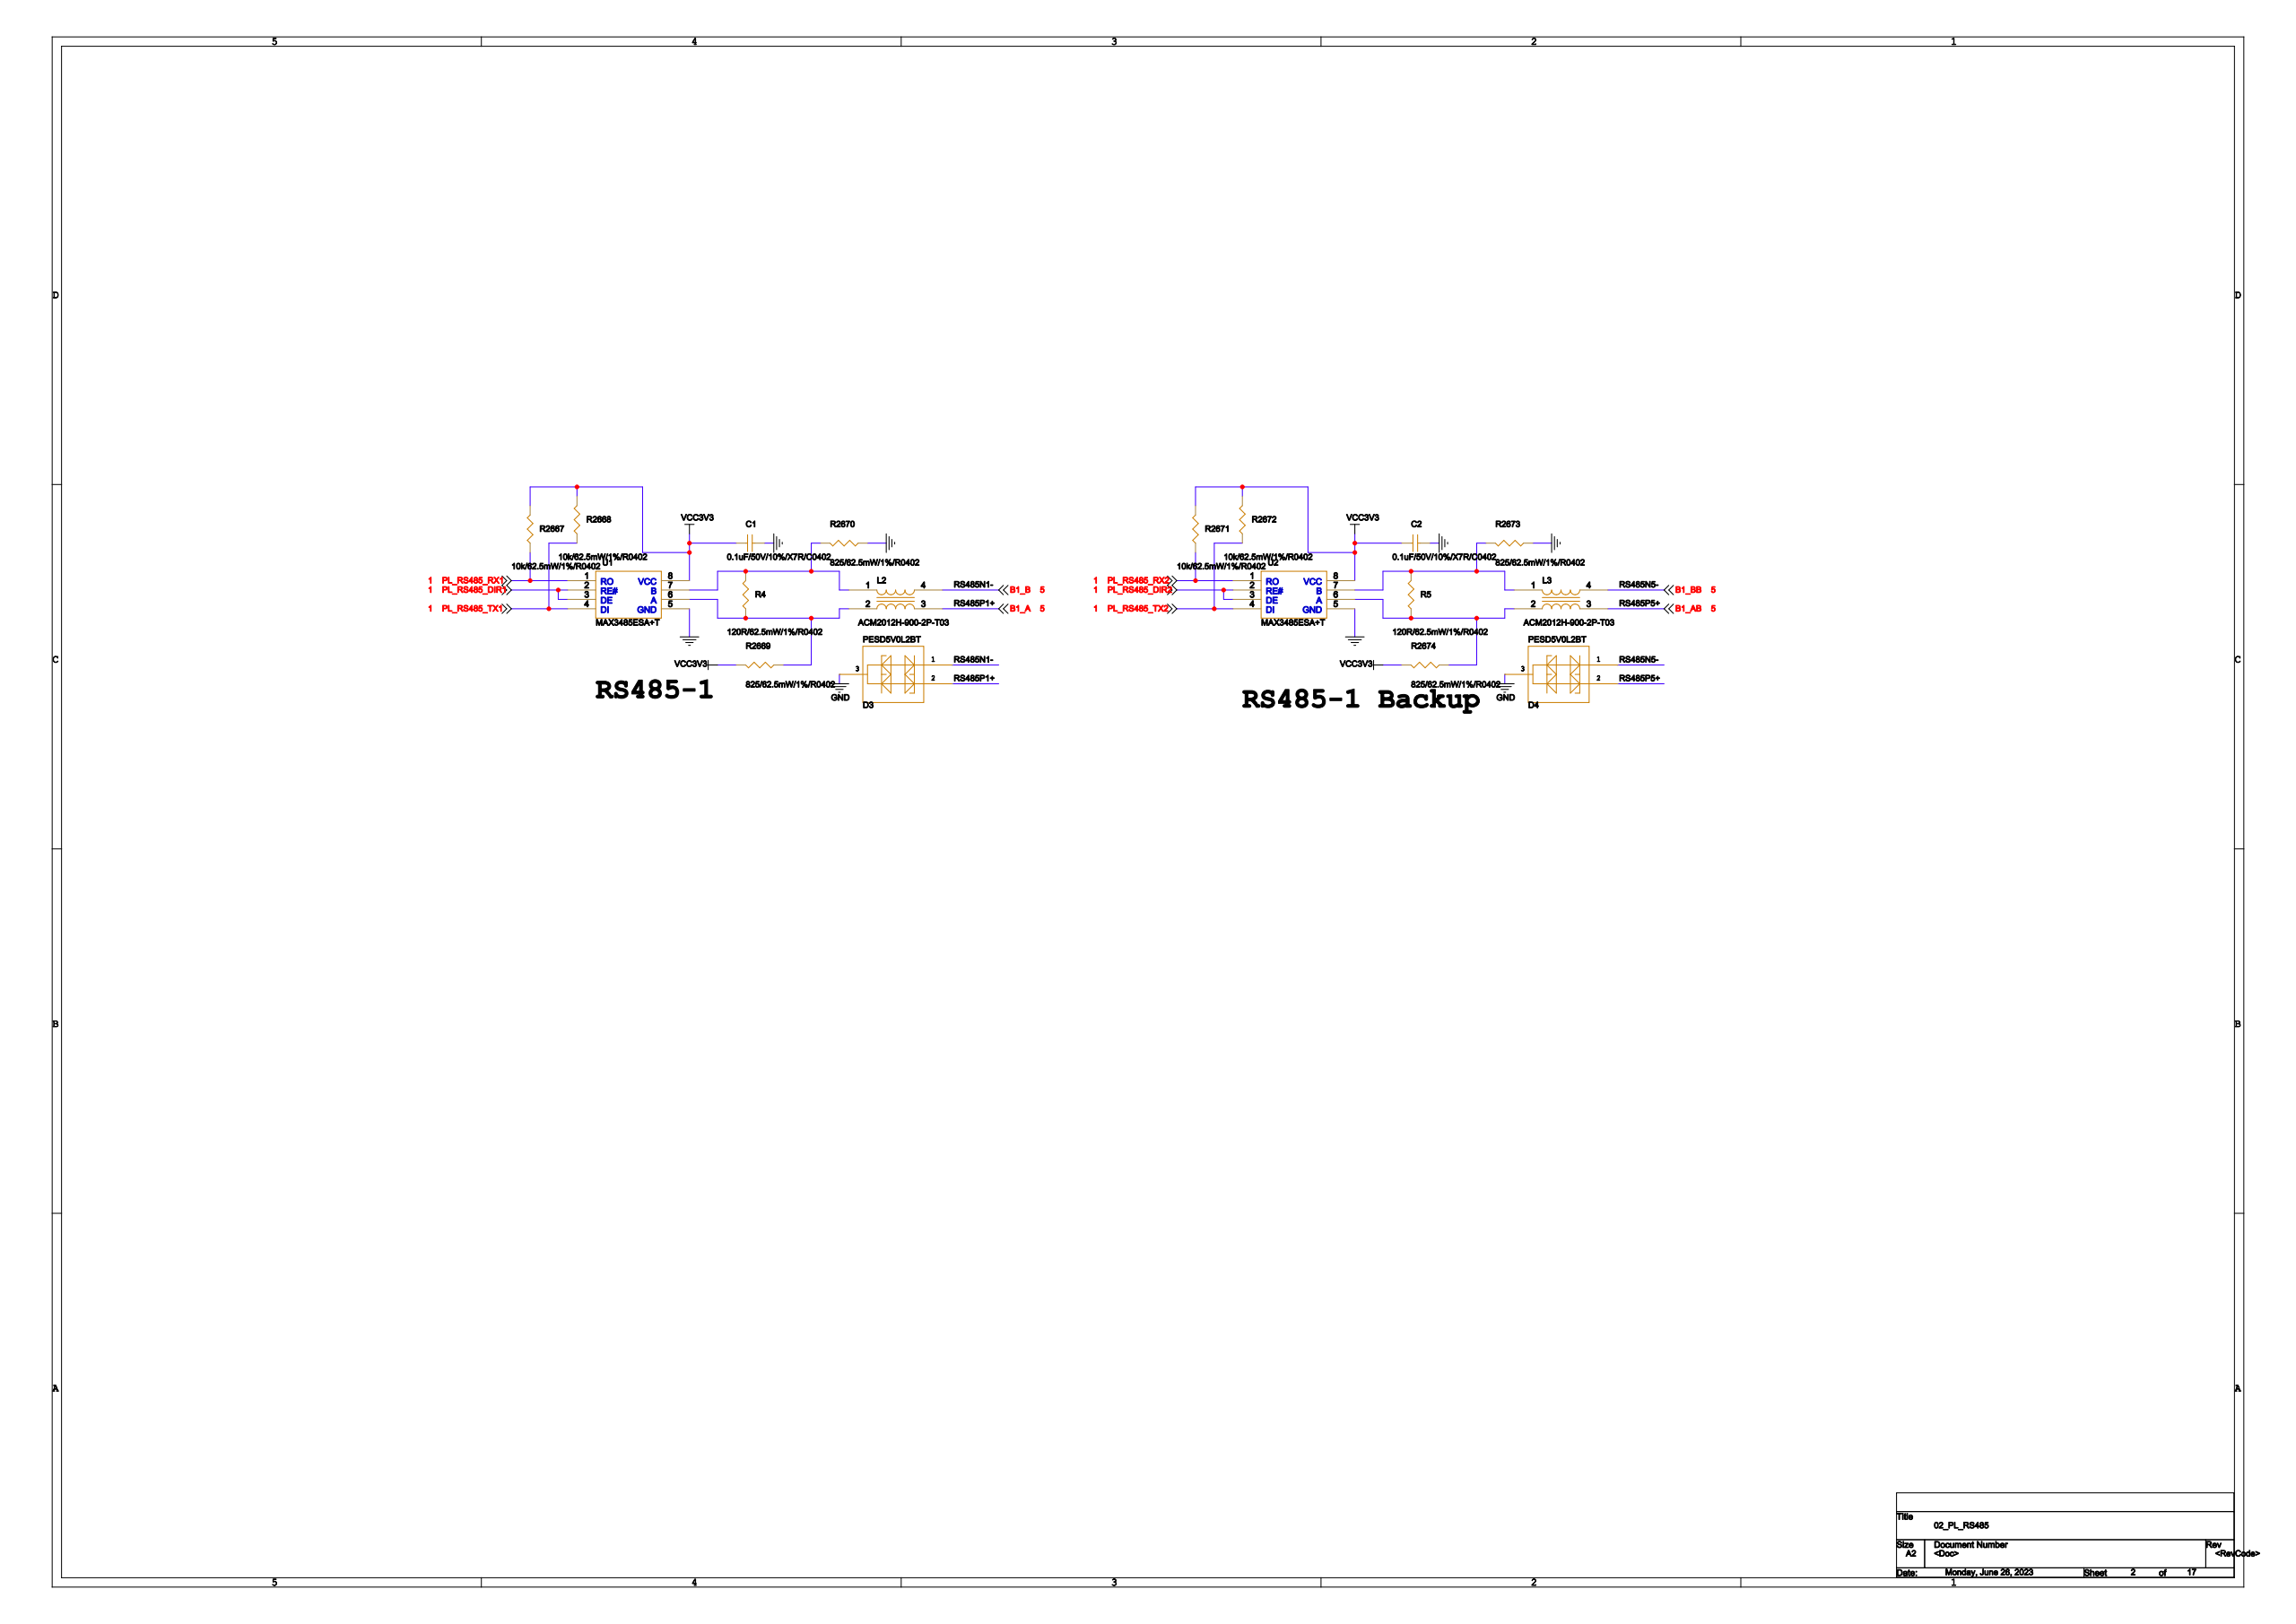Circuit board | Cadence Allegro | 2002 parts | 1538 nets | one sheet of the schematic
Parts on this sheet (reference | value | footprint):
C1 | 0.1uF/50V/10%/X7R/C0402 | 0402
C2 | 0.1uF/50V/10%/X7R/C0402 | 0402
D3 | PESD5V0L2BT | SOT23
D4 | PESD5V0L2BT | SOT23
L2 | ACM2012H-900-2P-T03 | ACM2012
L3 | ACM2012H-900-2P-T03 | ACM2012
R4 | 120R/62.5mW/1%/R0402 | 0402
R5 | 120R/62.5mW/1%/R0402 | 0402
R2667 | 10K/62.5mW/1%/R0402 | 0402
R2668 | 10K/62.5mW/1%/R0402 | 0402
R2669 | 825/62.5mW/1%/R0402 | 0402
R2670 | 825/62.5mW/1%/R0402 | 0402
R2671 | 10K/62.5mW/1%/R0402 | 0402
R2672 | 10K/62.5mW/1%/R0402 | 0402
R2673 | 825/62.5mW/1%/R0402 | 0402
R2674 | 825/62.5mW/1%/R0402 | 0402
U1 | MAX3485ESA+T | SO8
U2 | MAX3485ESA+T | SO8
Nets of these parts (net: part-pin ...):
3.3V: C1-1 C2-1 R2667-1 R2668-1 R2669-1 R2671-1 R2672-1 R2674-1 U1-8 U2-8
N21786216: L2-2 R4-2 R2669-2 U1-6
N21786207: L2-1 R4-1 R2670-1 U1-7
AGND: C1-2 C2-2 D3-3 D4-3 R2670-2 R2673-2 U1-5 U2-5
N23300009: L3-1 R5-1 R2673-1 U2-7
N23300015: L3-2 R5-2 R2674-2 U2-6
PL_RS485_TX1: R2668-2 U1-4
PL_RS485_DIR1: U1-2 U1-3
PL_RS485_RX1: R2667-2 U1-1
PL_RS485_TX2: R2672-2 U2-4
PL_RS485_DIR2: U2-2 U2-3
PL_RS485_RX2: R2671-2 U2-1
B1_A: D3-2 L2-3
B1_B: D3-1 L2-4
B1_AB: D4-2 L3-3
B1_BB: D4-1 L3-4